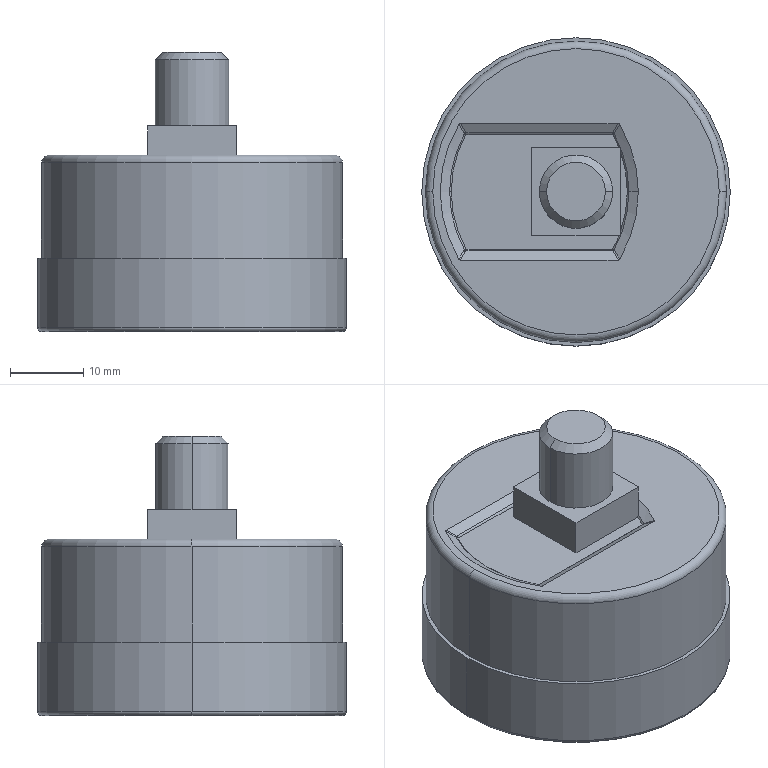Part | STEP file | 001. Pressure gauge (without flange) | 1 solid | 448 faces | box 42 x 42 x 38 mm | volume 32331 mm3 | plane 378 | spline 44 | cylinder 10 | torus 9 | cone 7 | commonest cylinder face diameters 1 x2 10 x2 35 x2 41 x2 42 x2